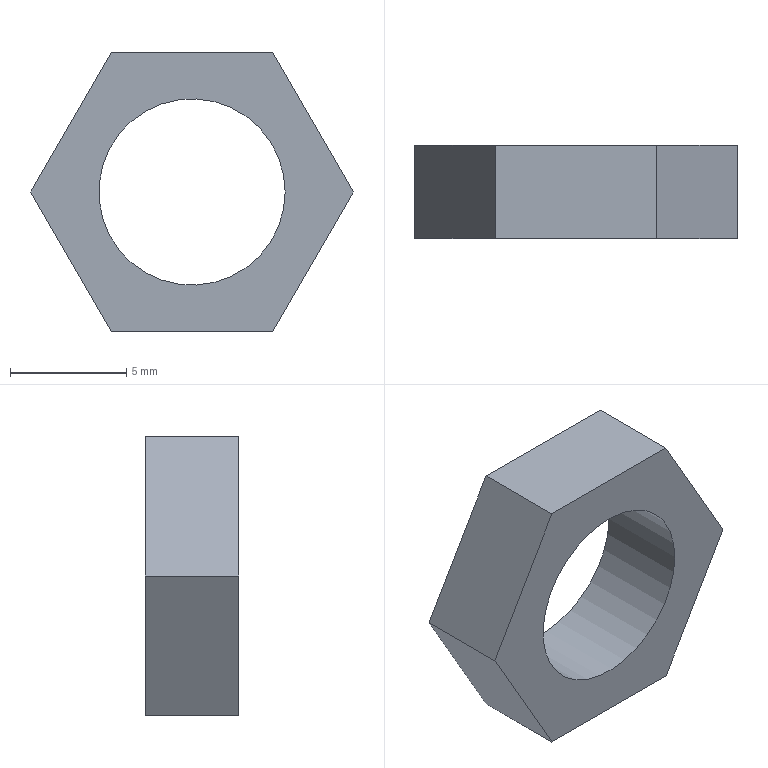Part | STEP file | 1-11.4 | 1 solid | 9 faces | box 13.856 x 4 x 12 mm | volume 297.769 mm3 | plane 8 | cylinder 1 | commonest cylinder face diameters 8 x1
STEP:
#1=CARTESIAN_POINT('',(0.,0.,0.));
#2=DIRECTION('',(0.,0.,1.));
#3=DIRECTION('',(1.,0.,0.));
#4=AXIS2_PLACEMENT_3D('',#1,#2,#3);
#5=CARTESIAN_POINT('',(6.928,0.,0.));
#6=VERTEX_POINT('',#5);
#7=CARTESIAN_POINT('',(3.464,0.,6.));
#8=VERTEX_POINT('',#7);
#9=CARTESIAN_POINT('',(6.928,0.,0.));
#10=DIRECTION('',(-0.5,0.,0.866));
#11=VECTOR('',#10,1.);
#12=LINE('',#9,#11);
#13=CARTESIAN_POINT('',(0.,0.,0.9282));
#14=DIRECTION('',(0.,-1.,0.));
#15=DIRECTION('',(1.,0.,0.));
#16=AXIS2_PLACEMENT_3D('',#13,#14,#15);
#17=PLANE('',#16);
#18=CARTESIAN_POINT('',(6.928,-0.9282));
#19=DIRECTION('',(-0.5,0.866));
#20=VECTOR('',#19,1.);
#21=LINE('',#18,#20);
#22=(GEOMETRIC_REPRESENTATION_CONTEXT(2)PARAMETRIC_REPRESENTATION_CONTEXT()REPRESENTATION_CONTEXT('',''));
#23=DEFINITIONAL_REPRESENTATION('',(#21),#22);
#24=PCURVE('',#17,#23);
#25=CARTESIAN_POINT('',(5.196,-2.,3.));
#26=DIRECTION('',(0.866,0.,0.5));
#27=DIRECTION('',(-0.5,0.,0.866));
#28=AXIS2_PLACEMENT_3D('',#25,#26,#27);
#29=PLANE('',#28);
#30=CARTESIAN_POINT('',(-3.464,-2.));
#31=DIRECTION('',(1.,0.));
#32=VECTOR('',#31,1.);
#33=LINE('',#30,#32);
#34=(GEOMETRIC_REPRESENTATION_CONTEXT(2)PARAMETRIC_REPRESENTATION_CONTEXT()REPRESENTATION_CONTEXT('',''));
#35=DEFINITIONAL_REPRESENTATION('',(#33),#34);
#36=PCURVE('',#29,#35);
#37=SURFACE_CURVE('',#12,(#24,#36),.PCURVE_S1.);
#38=EDGE_CURVE('',#6,#8,#37,.T.);
#39=ORIENTED_EDGE('',*,*,#38,.T.);
#40=CARTESIAN_POINT('',(-3.464,0.,6.));
#41=VERTEX_POINT('',#40);
#42=CARTESIAN_POINT('',(3.464,0.,6.));
#43=DIRECTION('',(-1.,0.,0.));
#44=VECTOR('',#43,1.);
#45=LINE('',#42,#44);
#46=CARTESIAN_POINT('',(3.464,5.072));
#47=DIRECTION('',(-1.,0.));
#48=VECTOR('',#47,1.);
#49=LINE('',#46,#48);
#50=(GEOMETRIC_REPRESENTATION_CONTEXT(2)PARAMETRIC_REPRESENTATION_CONTEXT()REPRESENTATION_CONTEXT('',''));
#51=DEFINITIONAL_REPRESENTATION('',(#49),#50);
#52=PCURVE('',#17,#51);
#53=CARTESIAN_POINT('',(0.,-2.,6.));
#54=DIRECTION('',(0.,0.,1.));
#55=DIRECTION('',(-1.,0.,0.));
#56=AXIS2_PLACEMENT_3D('',#53,#54,#55);
#57=PLANE('',#56);
#58=CARTESIAN_POINT('',(-3.464,-2.));
#59=DIRECTION('',(1.,0.));
#60=VECTOR('',#59,1.);
#61=LINE('',#58,#60);
#62=(GEOMETRIC_REPRESENTATION_CONTEXT(2)PARAMETRIC_REPRESENTATION_CONTEXT()REPRESENTATION_CONTEXT('',''));
#63=DEFINITIONAL_REPRESENTATION('',(#61),#62);
#64=PCURVE('',#57,#63);
#65=SURFACE_CURVE('',#45,(#52,#64),.PCURVE_S1.);
#66=EDGE_CURVE('',#8,#41,#65,.T.);
#67=ORIENTED_EDGE('',*,*,#66,.T.);
#68=CARTESIAN_POINT('',(-6.928,0.,0.));
#69=VERTEX_POINT('',#68);
#70=CARTESIAN_POINT('',(-3.464,0.,6.));
#71=DIRECTION('',(-0.5,0.,-0.866));
#72=VECTOR('',#71,1.);
#73=LINE('',#70,#72);
#74=CARTESIAN_POINT('',(-3.464,5.072));
#75=DIRECTION('',(-0.5,-0.866));
#76=VECTOR('',#75,1.);
#77=LINE('',#74,#76);
#78=(GEOMETRIC_REPRESENTATION_CONTEXT(2)PARAMETRIC_REPRESENTATION_CONTEXT()REPRESENTATION_CONTEXT('',''));
#79=DEFINITIONAL_REPRESENTATION('',(#77),#78);
#80=PCURVE('',#17,#79);
#81=CARTESIAN_POINT('',(-5.196,-2.,3.));
#82=DIRECTION('',(-0.866,0.,0.5));
#83=DIRECTION('',(-0.5,0.,-0.866));
#84=AXIS2_PLACEMENT_3D('',#81,#82,#83);
#85=PLANE('',#84);
#86=CARTESIAN_POINT('',(-3.464,-2.));
#87=DIRECTION('',(1.,0.));
#88=VECTOR('',#87,1.);
#89=LINE('',#86,#88);
#90=(GEOMETRIC_REPRESENTATION_CONTEXT(2)PARAMETRIC_REPRESENTATION_CONTEXT()REPRESENTATION_CONTEXT('',''));
#91=DEFINITIONAL_REPRESENTATION('',(#89),#90);
#92=PCURVE('',#85,#91);
#93=SURFACE_CURVE('',#73,(#80,#92),.PCURVE_S1.);
#94=EDGE_CURVE('',#41,#69,#93,.T.);
#95=ORIENTED_EDGE('',*,*,#94,.T.);
#96=CARTESIAN_POINT('',(-3.464,0.,-6.));
#97=VERTEX_POINT('',#96);
#98=CARTESIAN_POINT('',(-6.928,0.,0.));
#99=DIRECTION('',(0.5,0.,-0.866));
#100=VECTOR('',#99,1.);
#101=LINE('',#98,#100);
#102=CARTESIAN_POINT('',(-6.928,-0.9282));
#103=DIRECTION('',(0.5,-0.866));
#104=VECTOR('',#103,1.);
#105=LINE('',#102,#104);
#106=(GEOMETRIC_REPRESENTATION_CONTEXT(2)PARAMETRIC_REPRESENTATION_CONTEXT()REPRESENTATION_CONTEXT('',''));
#107=DEFINITIONAL_REPRESENTATION('',(#105),#106);
#108=PCURVE('',#17,#107);
#109=CARTESIAN_POINT('',(-5.196,-2.,-3.));
#110=DIRECTION('',(-0.866,0.,-0.5));
#111=DIRECTION('',(0.5,0.,-0.866));
#112=AXIS2_PLACEMENT_3D('',#109,#110,#111);
#113=PLANE('',#112);
#114=CARTESIAN_POINT('',(-3.464,-2.));
#115=DIRECTION('',(1.,0.));
#116=VECTOR('',#115,1.);
#117=LINE('',#114,#116);
#118=(GEOMETRIC_REPRESENTATION_CONTEXT(2)PARAMETRIC_REPRESENTATION_CONTEXT()REPRESENTATION_CONTEXT('',''));
#119=DEFINITIONAL_REPRESENTATION('',(#117),#118);
#120=PCURVE('',#113,#119);
#121=SURFACE_CURVE('',#101,(#108,#120),.PCURVE_S1.);
#122=EDGE_CURVE('',#69,#97,#121,.T.);
#123=ORIENTED_EDGE('',*,*,#122,.T.);
#124=CARTESIAN_POINT('',(3.464,0.,-6.));
#125=VERTEX_POINT('',#124);
#126=CARTESIAN_POINT('',(-3.464,0.,-6.));
#127=DIRECTION('',(1.,0.,0.));
#128=VECTOR('',#127,1.);
#129=LINE('',#126,#128);
#130=CARTESIAN_POINT('',(-3.464,-6.928));
#131=DIRECTION('',(1.,0.));
#132=VECTOR('',#131,1.);
#133=LINE('',#130,#132);
#134=(GEOMETRIC_REPRESENTATION_CONTEXT(2)PARAMETRIC_REPRESENTATION_CONTEXT()REPRESENTATION_CONTEXT('',''));
#135=DEFINITIONAL_REPRESENTATION('',(#133),#134);
#136=PCURVE('',#17,#135);
#137=CARTESIAN_POINT('',(0.,-2.,-6.));
#138=DIRECTION('',(0.,0.,-1.));
#139=DIRECTION('',(1.,0.,0.));
#140=AXIS2_PLACEMENT_3D('',#137,#138,#139);
#141=PLANE('',#140);
#142=CARTESIAN_POINT('',(-3.464,-2.));
#143=DIRECTION('',(1.,0.));
#144=VECTOR('',#143,1.);
#145=LINE('',#142,#144);
#146=(GEOMETRIC_REPRESENTATION_CONTEXT(2)PARAMETRIC_REPRESENTATION_CONTEXT()REPRESENTATION_CONTEXT('',''));
#147=DEFINITIONAL_REPRESENTATION('',(#145),#146);
#148=PCURVE('',#141,#147);
#149=SURFACE_CURVE('',#129,(#136,#148),.PCURVE_S1.);
#150=EDGE_CURVE('',#97,#125,#149,.T.);
#151=ORIENTED_EDGE('',*,*,#150,.T.);
#152=CARTESIAN_POINT('',(3.464,0.,-6.));
#153=DIRECTION('',(0.5,0.,0.866));
#154=VECTOR('',#153,1.);
#155=LINE('',#152,#154);
#156=CARTESIAN_POINT('',(3.464,-6.928));
#157=DIRECTION('',(0.5,0.866));
#158=VECTOR('',#157,1.);
#159=LINE('',#156,#158);
#160=(GEOMETRIC_REPRESENTATION_CONTEXT(2)PARAMETRIC_REPRESENTATION_CONTEXT()REPRESENTATION_CONTEXT('',''));
#161=DEFINITIONAL_REPRESENTATION('',(#159),#160);
#162=PCURVE('',#17,#161);
#163=CARTESIAN_POINT('',(5.196,-2.,-3.));
#164=DIRECTION('',(0.866,0.,-0.5));
#165=DIRECTION('',(0.5,0.,0.866));
#166=AXIS2_PLACEMENT_3D('',#163,#164,#165);
#167=PLANE('',#166);
#168=CARTESIAN_POINT('',(-3.464,-2.));
#169=DIRECTION('',(1.,0.));
#170=VECTOR('',#169,1.);
#171=LINE('',#168,#170);
#172=(GEOMETRIC_REPRESENTATION_CONTEXT(2)PARAMETRIC_REPRESENTATION_CONTEXT()REPRESENTATION_CONTEXT('',''));
#173=DEFINITIONAL_REPRESENTATION('',(#171),#172);
#174=PCURVE('',#167,#173);
#175=SURFACE_CURVE('',#155,(#162,#174),.PCURVE_S1.);
#176=EDGE_CURVE('',#125,#6,#175,.T.);
#177=ORIENTED_EDGE('',*,*,#176,.T.);
#178=EDGE_LOOP('',(#39,#67,#95,#123,#151,#177));
#179=FACE_BOUND('',#178,.F.);
#180=CARTESIAN_POINT('',(4.,0.,0.));
#181=VERTEX_POINT('',#180);
#182=CARTESIAN_POINT('',(0.,0.,0.));
#183=DIRECTION('',(0.,1.,0.));
#184=DIRECTION('',(1.,0.,0.));
#185=AXIS2_PLACEMENT_3D('',#182,#183,#184);
#186=CIRCLE('',#185,4.);
#187=CARTESIAN_POINT('',(4.,-0.9282));
#188=CARTESIAN_POINT('',(4.,-7.856));
#189=CARTESIAN_POINT('',(-2.,-4.392));
#190=CARTESIAN_POINT('',(-8.,-0.9282));
#191=CARTESIAN_POINT('',(-2.,2.536));
#192=CARTESIAN_POINT('',(4.,6.));
#193=CARTESIAN_POINT('',(4.,-0.9282));
#194=(BOUNDED_CURVE()B_SPLINE_CURVE(2,(#187,#188,#189,#190,#191,#192,#193),.UNSPECIFIED.,.T.,.F.)B_SPLINE_CURVE_WITH_KNOTS((1,2,2,2,2,1),(-2.094,0.,2.094,4.189,6.283,8.378),.UNSPECIFIED.)CURVE()GEOMETRIC_REPRESENTATION_ITEM()RATIONAL_B_SPLINE_CURVE((1.,0.5,1.,0.5,1.,0.5,1.))REPRESENTATION_ITEM(''));
#195=(GEOMETRIC_REPRESENTATION_CONTEXT(2)PARAMETRIC_REPRESENTATION_CONTEXT()REPRESENTATION_CONTEXT('',''));
#196=DEFINITIONAL_REPRESENTATION('',(#194),#195);
#197=PCURVE('',#17,#196);
#198=CARTESIAN_POINT('',(0.,0.,0.));
#199=DIRECTION('',(0.,-1.,0.));
#200=DIRECTION('',(1.,0.,0.));
#201=AXIS2_PLACEMENT_3D('',#198,#199,#200);
#202=CYLINDRICAL_SURFACE('',#201,4.);
#203=CARTESIAN_POINT('',(6.283,0.));
#204=DIRECTION('',(-1.,0.));
#205=VECTOR('',#204,1.);
#206=LINE('',#203,#205);
#207=(GEOMETRIC_REPRESENTATION_CONTEXT(2)PARAMETRIC_REPRESENTATION_CONTEXT()REPRESENTATION_CONTEXT('',''));
#208=DEFINITIONAL_REPRESENTATION('',(#206),#207);
#209=PCURVE('',#202,#208);
#210=SURFACE_CURVE('',#186,(#197,#209),.PCURVE_S1.);
#211=EDGE_CURVE('',#181,#181,#210,.T.);
#212=ORIENTED_EDGE('',*,*,#211,.T.);
#213=EDGE_LOOP('',(#212));
#214=FACE_BOUND('',#213,.F.);
#215=ADVANCED_FACE('',(#179,#214),#17,.F.);
#216=CARTESIAN_POINT('',(6.928,-4.,0.));
#217=VERTEX_POINT('',#216);
#218=CARTESIAN_POINT('',(3.464,-4.,6.));
#219=VERTEX_POINT('',#218);
#220=CARTESIAN_POINT('',(6.928,-4.,0.));
#221=DIRECTION('',(-0.5,0.,0.866));
#222=VECTOR('',#221,1.);
#223=LINE('',#220,#222);
#224=CARTESIAN_POINT('',(0.,-4.,0.9282));
#225=DIRECTION('',(0.,-1.,0.));
#226=DIRECTION('',(1.,0.,0.));
#227=AXIS2_PLACEMENT_3D('',#224,#225,#226);
#228=PLANE('',#227);
#229=CARTESIAN_POINT('',(6.928,-0.9282));
#230=DIRECTION('',(-0.5,0.866));
#231=VECTOR('',#230,1.);
#232=LINE('',#229,#231);
#233=(GEOMETRIC_REPRESENTATION_CONTEXT(2)PARAMETRIC_REPRESENTATION_CONTEXT()REPRESENTATION_CONTEXT('',''));
#234=DEFINITIONAL_REPRESENTATION('',(#232),#233);
#235=PCURVE('',#228,#234);
#236=CARTESIAN_POINT('',(-3.464,2.));
#237=DIRECTION('',(1.,0.));
#238=VECTOR('',#237,1.);
#239=LINE('',#236,#238);
#240=(GEOMETRIC_REPRESENTATION_CONTEXT(2)PARAMETRIC_REPRESENTATION_CONTEXT()REPRESENTATION_CONTEXT('',''));
#241=DEFINITIONAL_REPRESENTATION('',(#239),#240);
#242=PCURVE('',#29,#241);
#243=SURFACE_CURVE('',#223,(#235,#242),.PCURVE_S1.);
#244=EDGE_CURVE('',#217,#219,#243,.T.);
#245=ORIENTED_EDGE('',*,*,#244,.T.);
#246=CARTESIAN_POINT('',(-3.464,-4.,6.));
#247=VERTEX_POINT('',#246);
#248=CARTESIAN_POINT('',(3.464,-4.,6.));
#249=DIRECTION('',(-1.,0.,0.));
#250=VECTOR('',#249,1.);
#251=LINE('',#248,#250);
#252=CARTESIAN_POINT('',(3.464,5.072));
#253=DIRECTION('',(-1.,0.));
#254=VECTOR('',#253,1.);
#255=LINE('',#252,#254);
#256=(GEOMETRIC_REPRESENTATION_CONTEXT(2)PARAMETRIC_REPRESENTATION_CONTEXT()REPRESENTATION_CONTEXT('',''));
#257=DEFINITIONAL_REPRESENTATION('',(#255),#256);
#258=PCURVE('',#228,#257);
#259=CARTESIAN_POINT('',(-3.464,2.));
#260=DIRECTION('',(1.,0.));
#261=VECTOR('',#260,1.);
#262=LINE('',#259,#261);
#263=(GEOMETRIC_REPRESENTATION_CONTEXT(2)PARAMETRIC_REPRESENTATION_CONTEXT()REPRESENTATION_CONTEXT('',''));
#264=DEFINITIONAL_REPRESENTATION('',(#262),#263);
#265=PCURVE('',#57,#264);
#266=SURFACE_CURVE('',#251,(#258,#265),.PCURVE_S1.);
#267=EDGE_CURVE('',#219,#247,#266,.T.);
#268=ORIENTED_EDGE('',*,*,#267,.T.);
#269=CARTESIAN_POINT('',(-6.928,-4.,0.));
#270=VERTEX_POINT('',#269);
#271=CARTESIAN_POINT('',(-3.464,-4.,6.));
#272=DIRECTION('',(-0.5,0.,-0.866));
#273=VECTOR('',#272,1.);
#274=LINE('',#271,#273);
#275=CARTESIAN_POINT('',(-3.464,5.072));
#276=DIRECTION('',(-0.5,-0.866));
#277=VECTOR('',#276,1.);
#278=LINE('',#275,#277);
#279=(GEOMETRIC_REPRESENTATION_CONTEXT(2)PARAMETRIC_REPRESENTATION_CONTEXT()REPRESENTATION_CONTEXT('',''));
#280=DEFINITIONAL_REPRESENTATION('',(#278),#279);
#281=PCURVE('',#228,#280);
#282=CARTESIAN_POINT('',(-3.464,2.));
#283=DIRECTION('',(1.,0.));
#284=VECTOR('',#283,1.);
#285=LINE('',#282,#284);
#286=(GEOMETRIC_REPRESENTATION_CONTEXT(2)PARAMETRIC_REPRESENTATION_CONTEXT()REPRESENTATION_CONTEXT('',''));
#287=DEFINITIONAL_REPRESENTATION('',(#285),#286);
#288=PCURVE('',#85,#287);
#289=SURFACE_CURVE('',#274,(#281,#288),.PCURVE_S1.);
#290=EDGE_CURVE('',#247,#270,#289,.T.);
#291=ORIENTED_EDGE('',*,*,#290,.T.);
#292=CARTESIAN_POINT('',(-3.464,-4.,-6.));
#293=VERTEX_POINT('',#292);
#294=CARTESIAN_POINT('',(-6.928,-4.,0.));
#295=DIRECTION('',(0.5,0.,-0.866));
#296=VECTOR('',#295,1.);
#297=LINE('',#294,#296);
#298=CARTESIAN_POINT('',(-6.928,-0.9282));
#299=DIRECTION('',(0.5,-0.866));
#300=VECTOR('',#299,1.);
#301=LINE('',#298,#300);
#302=(GEOMETRIC_REPRESENTATION_CONTEXT(2)PARAMETRIC_REPRESENTATION_CONTEXT()REPRESENTATION_CONTEXT('',''));
#303=DEFINITIONAL_REPRESENTATION('',(#301),#302);
#304=PCURVE('',#228,#303);
#305=CARTESIAN_POINT('',(-3.464,2.));
#306=DIRECTION('',(1.,0.));
#307=VECTOR('',#306,1.);
#308=LINE('',#305,#307);
#309=(GEOMETRIC_REPRESENTATION_CONTEXT(2)PARAMETRIC_REPRESENTATION_CONTEXT()REPRESENTATION_CONTEXT('',''));
#310=DEFINITIONAL_REPRESENTATION('',(#308),#309);
#311=PCURVE('',#113,#310);
#312=SURFACE_CURVE('',#297,(#304,#311),.PCURVE_S1.);
#313=EDGE_CURVE('',#270,#293,#312,.T.);
#314=ORIENTED_EDGE('',*,*,#313,.T.);
#315=CARTESIAN_POINT('',(3.464,-4.,-6.));
#316=VERTEX_POINT('',#315);
#317=CARTESIAN_POINT('',(-3.464,-4.,-6.));
#318=DIRECTION('',(1.,0.,0.));
#319=VECTOR('',#318,1.);
#320=LINE('',#317,#319);
#321=CARTESIAN_POINT('',(-3.464,-6.928));
#322=DIRECTION('',(1.,0.));
#323=VECTOR('',#322,1.);
#324=LINE('',#321,#323);
#325=(GEOMETRIC_REPRESENTATION_CONTEXT(2)PARAMETRIC_REPRESENTATION_CONTEXT()REPRESENTATION_CONTEXT('',''));
#326=DEFINITIONAL_REPRESENTATION('',(#324),#325);
#327=PCURVE('',#228,#326);
#328=CARTESIAN_POINT('',(-3.464,2.));
#329=DIRECTION('',(1.,0.));
#330=VECTOR('',#329,1.);
#331=LINE('',#328,#330);
#332=(GEOMETRIC_REPRESENTATION_CONTEXT(2)PARAMETRIC_REPRESENTATION_CONTEXT()REPRESENTATION_CONTEXT('',''));
#333=DEFINITIONAL_REPRESENTATION('',(#331),#332);
#334=PCURVE('',#141,#333);
#335=SURFACE_CURVE('',#320,(#327,#334),.PCURVE_S1.);
#336=EDGE_CURVE('',#293,#316,#335,.T.);
#337=ORIENTED_EDGE('',*,*,#336,.T.);
#338=CARTESIAN_POINT('',(3.464,-4.,-6.));
#339=DIRECTION('',(0.5,0.,0.866));
#340=VECTOR('',#339,1.);
#341=LINE('',#338,#340);
#342=CARTESIAN_POINT('',(3.464,-6.928));
#343=DIRECTION('',(0.5,0.866));
#344=VECTOR('',#343,1.);
#345=LINE('',#342,#344);
#346=(GEOMETRIC_REPRESENTATION_CONTEXT(2)PARAMETRIC_REPRESENTATION_CONTEXT()REPRESENTATION_CONTEXT('',''));
#347=DEFINITIONAL_REPRESENTATION('',(#345),#346);
#348=PCURVE('',#228,#347);
#349=CARTESIAN_POINT('',(-3.464,2.));
#350=DIRECTION('',(1.,0.));
#351=VECTOR('',#350,1.);
#352=LINE('',#349,#351);
#353=(GEOMETRIC_REPRESENTATION_CONTEXT(2)PARAMETRIC_REPRESENTATION_CONTEXT()REPRESENTATION_CONTEXT('',''));
#354=DEFINITIONAL_REPRESENTATION('',(#352),#353);
#355=PCURVE('',#167,#354);
#356=SURFACE_CURVE('',#341,(#348,#355),.PCURVE_S1.);
#357=EDGE_CURVE('',#316,#217,#356,.T.);
#358=ORIENTED_EDGE('',*,*,#357,.T.);
#359=EDGE_LOOP('',(#245,#268,#291,#314,#337,#358));
#360=FACE_BOUND('',#359,.T.);
#361=CARTESIAN_POINT('',(4.,-4.,0.));
#362=VERTEX_POINT('',#361);
#363=CARTESIAN_POINT('',(0.,-4.,0.));
#364=DIRECTION('',(0.,1.,0.));
#365=DIRECTION('',(1.,0.,0.));
#366=AXIS2_PLACEMENT_3D('',#363,#364,#365);
#367=CIRCLE('',#366,4.);
#368=CARTESIAN_POINT('',(4.,-0.9282));
#369=CARTESIAN_POINT('',(4.,-7.856));
#370=CARTESIAN_POINT('',(-2.,-4.392));
#371=CARTESIAN_POINT('',(-8.,-0.9282));
#372=CARTESIAN_POINT('',(-2.,2.536));
#373=CARTESIAN_POINT('',(4.,6.));
#374=CARTESIAN_POINT('',(4.,-0.9282));
#375=(BOUNDED_CURVE()B_SPLINE_CURVE(2,(#368,#369,#370,#371,#372,#373,#374),.UNSPECIFIED.,.T.,.F.)B_SPLINE_CURVE_WITH_KNOTS((1,2,2,2,2,1),(-2.094,0.,2.094,4.189,6.283,8.378),.UNSPECIFIED.)CURVE()GEOMETRIC_REPRESENTATION_ITEM()RATIONAL_B_SPLINE_CURVE((1.,0.5,1.,0.5,1.,0.5,1.))REPRESENTATION_ITEM(''));
#376=(GEOMETRIC_REPRESENTATION_CONTEXT(2)PARAMETRIC_REPRESENTATION_CONTEXT()REPRESENTATION_CONTEXT('',''));
#377=DEFINITIONAL_REPRESENTATION('',(#375),#376);
#378=PCURVE('',#228,#377);
#379=CARTESIAN_POINT('',(6.283,4.));
#380=DIRECTION('',(-1.,0.));
#381=VECTOR('',#380,1.);
#382=LINE('',#379,#381);
#383=(GEOMETRIC_REPRESENTATION_CONTEXT(2)PARAMETRIC_REPRESENTATION_CONTEXT()REPRESENTATION_CONTEXT('',''));
#384=DEFINITIONAL_REPRESENTATION('',(#382),#383);
#385=PCURVE('',#202,#384);
#386=SURFACE_CURVE('',#367,(#378,#385),.PCURVE_S1.);
#387=EDGE_CURVE('',#362,#362,#386,.T.);
#388=ORIENTED_EDGE('',*,*,#387,.T.);
#389=EDGE_LOOP('',(#388));
#390=FACE_BOUND('',#389,.T.);
#391=ADVANCED_FACE('',(#360,#390),#228,.T.);
#392=ORIENTED_EDGE('',*,*,#38,.T.);
#393=CARTESIAN_POINT('',(3.464,0.,6.));
#394=DIRECTION('',(0.,-1.,0.));
#395=VECTOR('',#394,1.);
#396=LINE('',#393,#395);
#397=CARTESIAN_POINT('',(3.464,-2.));
#398=DIRECTION('',(0.,1.));
#399=VECTOR('',#398,1.);
#400=LINE('',#397,#399);
#401=(GEOMETRIC_REPRESENTATION_CONTEXT(2)PARAMETRIC_REPRESENTATION_CONTEXT()REPRESENTATION_CONTEXT('',''));
#402=DEFINITIONAL_REPRESENTATION('',(#400),#401);
#403=PCURVE('',#29,#402);
#404=CARTESIAN_POINT('',(-3.464,-2.));
#405=DIRECTION('',(0.,1.));
#406=VECTOR('',#405,1.);
#407=LINE('',#404,#406);
#408=(GEOMETRIC_REPRESENTATION_CONTEXT(2)PARAMETRIC_REPRESENTATION_CONTEXT()REPRESENTATION_CONTEXT('',''));
#409=DEFINITIONAL_REPRESENTATION('',(#407),#408);
#410=PCURVE('',#57,#409);
#411=SURFACE_CURVE('',#396,(#403,#410),.PCURVE_S1.);
#412=EDGE_CURVE('',#8,#219,#411,.T.);
#413=ORIENTED_EDGE('',*,*,#412,.T.);
#414=ORIENTED_EDGE('',*,*,#244,.F.);
#415=CARTESIAN_POINT('',(6.928,0.,0.));
#416=DIRECTION('',(0.,-1.,0.));
#417=VECTOR('',#416,1.);
#418=LINE('',#415,#417);
#419=CARTESIAN_POINT('',(-3.464,-2.));
#420=DIRECTION('',(0.,1.));
#421=VECTOR('',#420,1.);
#422=LINE('',#419,#421);
#423=(GEOMETRIC_REPRESENTATION_CONTEXT(2)PARAMETRIC_REPRESENTATION_CONTEXT()REPRESENTATION_CONTEXT('',''));
#424=DEFINITIONAL_REPRESENTATION('',(#422),#423);
#425=PCURVE('',#29,#424);
#426=CARTESIAN_POINT('',(3.464,-2.));
#427=DIRECTION('',(0.,1.));
#428=VECTOR('',#427,1.);
#429=LINE('',#426,#428);
#430=(GEOMETRIC_REPRESENTATION_CONTEXT(2)PARAMETRIC_REPRESENTATION_CONTEXT()REPRESENTATION_CONTEXT('',''));
#431=DEFINITIONAL_REPRESENTATION('',(#429),#430);
#432=PCURVE('',#167,#431);
#433=SURFACE_CURVE('',#418,(#425,#432),.PCURVE_S1.);
#434=EDGE_CURVE('',#6,#217,#433,.T.);
#435=ORIENTED_EDGE('',*,*,#434,.F.);
#436=EDGE_LOOP('',(#392,#413,#414,#435));
#437=FACE_BOUND('',#436,.T.);
#438=ADVANCED_FACE('',(#437),#29,.T.);
#439=ORIENTED_EDGE('',*,*,#66,.T.);
#440=CARTESIAN_POINT('',(-3.464,0.,6.));
#441=DIRECTION('',(0.,-1.,0.));
#442=VECTOR('',#441,1.);
#443=LINE('',#440,#442);
#444=CARTESIAN_POINT('',(3.464,-2.));
#445=DIRECTION('',(0.,1.));
#446=VECTOR('',#445,1.);
#447=LINE('',#444,#446);
#448=(GEOMETRIC_REPRESENTATION_CONTEXT(2)PARAMETRIC_REPRESENTATION_CONTEXT()REPRESENTATION_CONTEXT('',''));
#449=DEFINITIONAL_REPRESENTATION('',(#447),#448);
#450=PCURVE('',#57,#449);
#451=CARTESIAN_POINT('',(-3.464,-2.));
#452=DIRECTION('',(0.,1.));
#453=VECTOR('',#452,1.);
#454=LINE('',#451,#453);
#455=(GEOMETRIC_REPRESENTATION_CONTEXT(2)PARAMETRIC_REPRESENTATION_CONTEXT()REPRESENTATION_CONTEXT('',''));
#456=DEFINITIONAL_REPRESENTATION('',(#454),#455);
#457=PCURVE('',#85,#456);
#458=SURFACE_CURVE('',#443,(#450,#457),.PCURVE_S1.);
#459=EDGE_CURVE('',#41,#247,#458,.T.);
#460=ORIENTED_EDGE('',*,*,#459,.T.);
#461=ORIENTED_EDGE('',*,*,#267,.F.);
#462=ORIENTED_EDGE('',*,*,#412,.F.);
#463=EDGE_LOOP('',(#439,#460,#461,#462));
#464=FACE_BOUND('',#463,.T.);
#465=ADVANCED_FACE('',(#464),#57,.T.);
#466=ORIENTED_EDGE('',*,*,#94,.T.);
#467=CARTESIAN_POINT('',(-6.928,0.,0.));
#468=DIRECTION('',(0.,-1.,0.));
#469=VECTOR('',#468,1.);
#470=LINE('',#467,#469);
#471=CARTESIAN_POINT('',(3.464,-2.));
#472=DIRECTION('',(0.,1.));
#473=VECTOR('',#472,1.);
#474=LINE('',#471,#473);
#475=(GEOMETRIC_REPRESENTATION_CONTEXT(2)PARAMETRIC_REPRESENTATION_CONTEXT()REPRESENTATION_CONTEXT('',''));
#476=DEFINITIONAL_REPRESENTATION('',(#474),#475);
#477=PCURVE('',#85,#476);
#478=CARTESIAN_POINT('',(-3.464,-2.));
#479=DIRECTION('',(0.,1.));
#480=VECTOR('',#479,1.);
#481=LINE('',#478,#480);
#482=(GEOMETRIC_REPRESENTATION_CONTEXT(2)PARAMETRIC_REPRESENTATION_CONTEXT()REPRESENTATION_CONTEXT('',''));
#483=DEFINITIONAL_REPRESENTATION('',(#481),#482);
#484=PCURVE('',#113,#483);
#485=SURFACE_CURVE('',#470,(#477,#484),.PCURVE_S1.);
#486=EDGE_CURVE('',#69,#270,#485,.T.);
#487=ORIENTED_EDGE('',*,*,#486,.T.);
#488=ORIENTED_EDGE('',*,*,#290,.F.);
#489=ORIENTED_EDGE('',*,*,#459,.F.);
#490=EDGE_LOOP('',(#466,#487,#488,#489));
#491=FACE_BOUND('',#490,.T.);
#492=ADVANCED_FACE('',(#491),#85,.T.);
#493=ORIENTED_EDGE('',*,*,#122,.T.);
#494=CARTESIAN_POINT('',(-3.464,0.,-6.));
#495=DIRECTION('',(0.,-1.,0.));
#496=VECTOR('',#495,1.);
#497=LINE('',#494,#496);
#498=CARTESIAN_POINT('',(3.464,-2.));
#499=DIRECTION('',(0.,1.));
#500=VECTOR('',#499,1.);
#501=LINE('',#498,#500);
#502=(GEOMETRIC_REPRESENTATION_CONTEXT(2)PARAMETRIC_REPRESENTATION_CONTEXT()REPRESENTATION_CONTEXT('',''));
#503=DEFINITIONAL_REPRESENTATION('',(#501),#502);
#504=PCURVE('',#113,#503);
#505=CARTESIAN_POINT('',(-3.464,-2.));
#506=DIRECTION('',(0.,1.));
#507=VECTOR('',#506,1.);
#508=LINE('',#505,#507);
#509=(GEOMETRIC_REPRESENTATION_CONTEXT(2)PARAMETRIC_REPRESENTATION_CONTEXT()REPRESENTATION_CONTEXT('',''));
#510=DEFINITIONAL_REPRESENTATION('',(#508),#509);
#511=PCURVE('',#141,#510);
#512=SURFACE_CURVE('',#497,(#504,#511),.PCURVE_S1.);
#513=EDGE_CURVE('',#97,#293,#512,.T.);
#514=ORIENTED_EDGE('',*,*,#513,.T.);
#515=ORIENTED_EDGE('',*,*,#313,.F.);
#516=ORIENTED_EDGE('',*,*,#486,.F.);
#517=EDGE_LOOP('',(#493,#514,#515,#516));
#518=FACE_BOUND('',#517,.T.);
#519=ADVANCED_FACE('',(#518),#113,.T.);
#520=ORIENTED_EDGE('',*,*,#150,.T.);
#521=CARTESIAN_POINT('',(3.464,0.,-6.));
#522=DIRECTION('',(0.,-1.,0.));
#523=VECTOR('',#522,1.);
#524=LINE('',#521,#523);
#525=CARTESIAN_POINT('',(3.464,-2.));
#526=DIRECTION('',(0.,1.));
#527=VECTOR('',#526,1.);
#528=LINE('',#525,#527);
#529=(GEOMETRIC_REPRESENTATION_CONTEXT(2)PARAMETRIC_REPRESENTATION_CONTEXT()REPRESENTATION_CONTEXT('',''));
#530=DEFINITIONAL_REPRESENTATION('',(#528),#529);
#531=PCURVE('',#141,#530);
#532=CARTESIAN_POINT('',(-3.464,-2.));
#533=DIRECTION('',(0.,1.));
#534=VECTOR('',#533,1.);
#535=LINE('',#532,#534);
#536=(GEOMETRIC_REPRESENTATION_CONTEXT(2)PARAMETRIC_REPRESENTATION_CONTEXT()REPRESENTATION_CONTEXT('',''));
#537=DEFINITIONAL_REPRESENTATION('',(#535),#536);
#538=PCURVE('',#167,#537);
#539=SURFACE_CURVE('',#524,(#531,#538),.PCURVE_S1.);
#540=EDGE_CURVE('',#125,#316,#539,.T.);
#541=ORIENTED_EDGE('',*,*,#540,.T.);
#542=ORIENTED_EDGE('',*,*,#336,.F.);
#543=ORIENTED_EDGE('',*,*,#513,.F.);
#544=EDGE_LOOP('',(#520,#541,#542,#543));
#545=FACE_BOUND('',#544,.T.);
#546=ADVANCED_FACE('',(#545),#141,.T.);
#547=ORIENTED_EDGE('',*,*,#176,.T.);
#548=ORIENTED_EDGE('',*,*,#434,.T.);
#549=ORIENTED_EDGE('',*,*,#357,.F.);
#550=ORIENTED_EDGE('',*,*,#540,.F.);
#551=EDGE_LOOP('',(#547,#548,#549,#550));
#552=FACE_BOUND('',#551,.T.);
#553=ADVANCED_FACE('',(#552),#167,.T.);
#554=CARTESIAN_POINT('',(4.,0.,0.));
#555=DIRECTION('',(0.,-1.,0.));
#556=VECTOR('',#555,1.);
#557=LINE('',#554,#556);
#558=CARTESIAN_POINT('',(6.283,0.));
#559=DIRECTION('',(0.,1.));
#560=VECTOR('',#559,1.);
#561=LINE('',#558,#560);
#562=(GEOMETRIC_REPRESENTATION_CONTEXT(2)PARAMETRIC_REPRESENTATION_CONTEXT()REPRESENTATION_CONTEXT('',''));
#563=DEFINITIONAL_REPRESENTATION('',(#561),#562);
#564=PCURVE('',#202,#563);
#565=CARTESIAN_POINT('',(0.,0.));
#566=DIRECTION('',(0.,1.));
#567=VECTOR('',#566,1.);
#568=LINE('',#565,#567);
#569=(GEOMETRIC_REPRESENTATION_CONTEXT(2)PARAMETRIC_REPRESENTATION_CONTEXT()REPRESENTATION_CONTEXT('',''));
#570=DEFINITIONAL_REPRESENTATION('',(#568),#569);
#571=PCURVE('',#202,#570);
#572=SEAM_CURVE('',#557,(#564,#571),.PCURVE_S1.);
#573=EDGE_CURVE('',#181,#362,#572,.T.);
#574=ORIENTED_EDGE('',*,*,#573,.T.);
#575=ORIENTED_EDGE('',*,*,#387,.T.);
#576=ORIENTED_EDGE('',*,*,#573,.F.);
#577=ORIENTED_EDGE('',*,*,#211,.F.);
#578=EDGE_LOOP('',(#574,#575,#576,#577));
#579=FACE_BOUND('',#578,.F.);
#580=ADVANCED_FACE('',(#579),#202,.F.);
#581=CLOSED_SHELL('',(#215,#391,#438,#465,#492,#519,#546,#553,#580));
#582=MANIFOLD_SOLID_BREP('',#581);
#583=(LENGTH_UNIT()NAMED_UNIT(*)SI_UNIT(.MILLI.,.METRE.));
#584=UNCERTAINTY_MEASURE_WITH_UNIT(LENGTH_MEASURE(0.0000001),#583,'','');
#585=(NAMED_UNIT(*)PLANE_ANGLE_UNIT()SI_UNIT($,.RADIAN.));
#586=(NAMED_UNIT(*)SI_UNIT($,.STERADIAN.)SOLID_ANGLE_UNIT());
#587=(GEOMETRIC_REPRESENTATION_CONTEXT(3)GLOBAL_UNCERTAINTY_ASSIGNED_CONTEXT((#584))GLOBAL_UNIT_ASSIGNED_CONTEXT((#583,#585,#586))REPRESENTATION_CONTEXT('',''));
#588=ADVANCED_BREP_SHAPE_REPRESENTATION('',(#4,#582),#587);